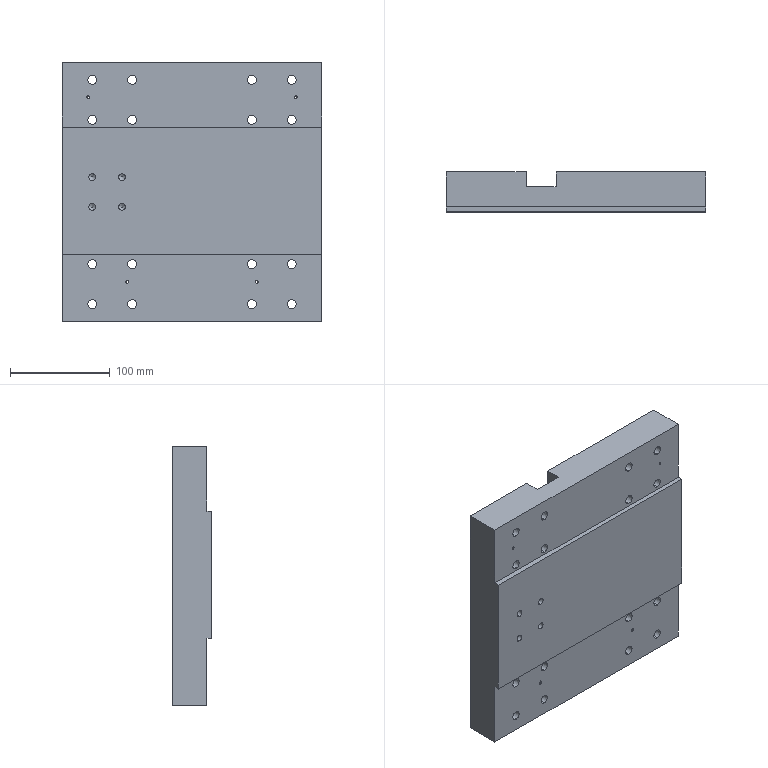Part | STEP file | Connecting Seat | 1 solid | 126 faces | box 260 x 40 x 260 mm | volume 2352118 mm3 | cylinder 80 | plane 30 | cone 16 | commonest cylinder face diameters 9 x32 14 x32 6.8 x8 10.2 x8